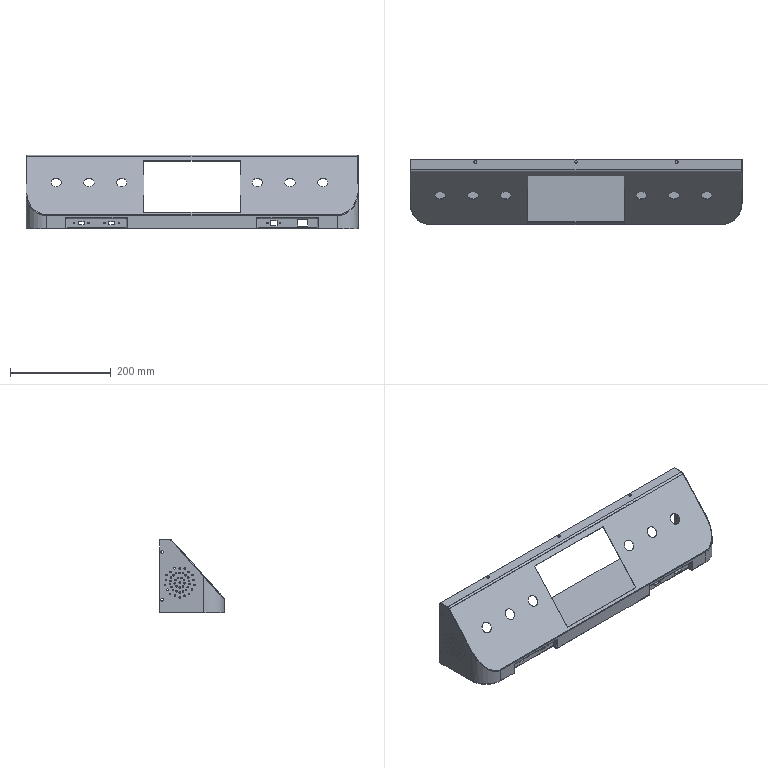Part | STEP file | 3 solids | 414 faces | box 660.4 x 129.2 x 145.9 mm | volume 256487 mm3 | cylinder 278 | plane 124 | spline 10 | torus 2 | commonest cylinder face diameters 3 x184 2 x21 4.5 x21 3.2 x12 22 x12 1.473 x8